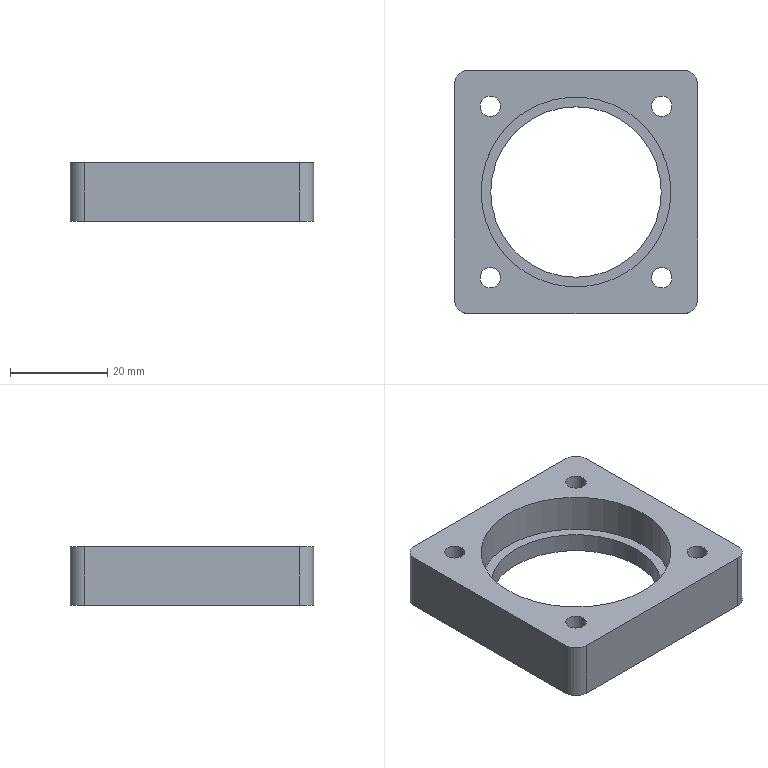Part | 1 solid | 23 faces | box 50 x 50 x 12 mm | volume 15837 mm3 | cylinder 16 | plane 7 | commonest cylinder face diameters 4.2 x8 6 x4 35 x2 39 x2
STEP:
#1=CARTESIAN_POINT('',(15.5,49.,-8.));
#2=VERTEX_POINT('',#1);
#3=CARTESIAN_POINT('',(54.5,49.,-8.));
#4=VERTEX_POINT('',#3);
#5=CARTESIAN_POINT('',(35.,49.,-8.));
#6=DIRECTION('',(0.,0.,1.));
#7=DIRECTION('',(1.,0.,0.));
#8=AXIS2_PLACEMENT_3D('',#5,#6,#7);
#9=CIRCLE('',#8,19.5);
#10=EDGE_CURVE('',#2,#4,#9,.T.);
#11=ORIENTED_EDGE('',*,*,#10,.F.);
#12=CARTESIAN_POINT('',(15.5,49.,0.));
#13=VERTEX_POINT('',#12);
#14=CARTESIAN_POINT('',(15.5,49.,-8.));
#15=DIRECTION('',(0.,0.,1.));
#16=VECTOR('',#15,1000.);
#17=LINE('',#14,#16);
#18=EDGE_CURVE('',#2,#13,#17,.T.);
#19=ORIENTED_EDGE('',*,*,#18,.T.);
#20=CARTESIAN_POINT('',(54.5,49.,0.));
#21=VERTEX_POINT('',#20);
#22=CARTESIAN_POINT('',(35.,49.,0.));
#23=DIRECTION('',(0.,0.,1.));
#24=DIRECTION('',(1.,0.,0.));
#25=AXIS2_PLACEMENT_3D('',#22,#23,#24);
#26=CIRCLE('',#25,19.5);
#27=EDGE_CURVE('',#13,#21,#26,.T.);
#28=ORIENTED_EDGE('',*,*,#27,.T.);
#29=CARTESIAN_POINT('',(54.5,49.,-8.));
#30=DIRECTION('',(0.,0.,1.));
#31=VECTOR('',#30,1000.);
#32=LINE('',#29,#31);
#33=EDGE_CURVE('',#4,#21,#32,.T.);
#34=ORIENTED_EDGE('',*,*,#33,.F.);
#35=EDGE_LOOP('',(#11,#19,#28,#34));
#36=FACE_OUTER_BOUND('',#35,.T.);
#37=CARTESIAN_POINT('',(35.,49.,-8.));
#38=DIRECTION('',(0.,0.,1.));
#39=DIRECTION('',(1.,0.,0.));
#40=AXIS2_PLACEMENT_3D('',#37,#38,#39);
#41=CYLINDRICAL_SURFACE('',#40,19.5);
#42=ADVANCED_FACE('',(#36),#41,.F.);
#43=CARTESIAN_POINT('',(19.497,66.604,-12.));
#44=VERTEX_POINT('',#43);
#45=CARTESIAN_POINT('',(15.297,66.604,-12.));
#46=VERTEX_POINT('',#45);
#47=CARTESIAN_POINT('',(17.397,66.604,-12.));
#48=DIRECTION('',(0.,0.,-1.));
#49=DIRECTION('',(1.,0.,0.));
#50=AXIS2_PLACEMENT_3D('',#47,#48,#49);
#51=CIRCLE('',#50,2.1);
#52=EDGE_CURVE('',#44,#46,#51,.T.);
#53=ORIENTED_EDGE('',*,*,#52,.T.);
#54=CARTESIAN_POINT('',(15.297,66.604,0.));
#55=VERTEX_POINT('',#54);
#56=CARTESIAN_POINT('',(15.297,66.604,0.));
#57=DIRECTION('',(0.,0.,1.));
#58=VECTOR('',#57,1000.);
#59=LINE('',#56,#58);
#60=EDGE_CURVE('',#46,#55,#59,.T.);
#61=ORIENTED_EDGE('',*,*,#60,.T.);
#62=CARTESIAN_POINT('',(19.497,66.604,0.));
#63=VERTEX_POINT('',#62);
#64=CARTESIAN_POINT('',(17.397,66.604,0.));
#65=DIRECTION('',(0.,0.,1.));
#66=DIRECTION('',(1.,0.,0.));
#67=AXIS2_PLACEMENT_3D('',#64,#65,#66);
#68=CIRCLE('',#67,2.1);
#69=EDGE_CURVE('',#55,#63,#68,.T.);
#70=ORIENTED_EDGE('',*,*,#69,.T.);
#71=CARTESIAN_POINT('',(19.497,66.604,0.));
#72=DIRECTION('',(0.,0.,1.));
#73=VECTOR('',#72,1000.);
#74=LINE('',#71,#73);
#75=EDGE_CURVE('',#44,#63,#74,.T.);
#76=ORIENTED_EDGE('',*,*,#75,.F.);
#77=EDGE_LOOP('',(#53,#61,#70,#76));
#78=FACE_OUTER_BOUND('',#77,.T.);
#79=CARTESIAN_POINT('',(17.397,66.604,0.));
#80=DIRECTION('',(0.,0.,1.));
#81=DIRECTION('',(1.,0.,0.));
#82=AXIS2_PLACEMENT_3D('',#79,#80,#81);
#83=CYLINDRICAL_SURFACE('',#82,2.1);
#84=ADVANCED_FACE('',(#78),#83,.F.);
#85=CARTESIAN_POINT('',(54.704,66.603,-12.));
#86=VERTEX_POINT('',#85);
#87=CARTESIAN_POINT('',(50.504,66.603,-12.));
#88=VERTEX_POINT('',#87);
#89=CARTESIAN_POINT('',(52.604,66.603,-12.));
#90=DIRECTION('',(0.,0.,-1.));
#91=DIRECTION('',(1.,0.,0.));
#92=AXIS2_PLACEMENT_3D('',#89,#90,#91);
#93=CIRCLE('',#92,2.1);
#94=EDGE_CURVE('',#86,#88,#93,.T.);
#95=ORIENTED_EDGE('',*,*,#94,.T.);
#96=CARTESIAN_POINT('',(50.504,66.603,0.));
#97=VERTEX_POINT('',#96);
#98=CARTESIAN_POINT('',(50.504,66.603,0.));
#99=DIRECTION('',(0.,0.,1.));
#100=VECTOR('',#99,1000.);
#101=LINE('',#98,#100);
#102=EDGE_CURVE('',#88,#97,#101,.T.);
#103=ORIENTED_EDGE('',*,*,#102,.T.);
#104=CARTESIAN_POINT('',(54.704,66.603,0.));
#105=VERTEX_POINT('',#104);
#106=CARTESIAN_POINT('',(52.604,66.603,0.));
#107=DIRECTION('',(0.,0.,1.));
#108=DIRECTION('',(1.,0.,0.));
#109=AXIS2_PLACEMENT_3D('',#106,#107,#108);
#110=CIRCLE('',#109,2.1);
#111=EDGE_CURVE('',#97,#105,#110,.T.);
#112=ORIENTED_EDGE('',*,*,#111,.T.);
#113=CARTESIAN_POINT('',(54.704,66.603,0.));
#114=DIRECTION('',(0.,0.,1.));
#115=VECTOR('',#114,1000.);
#116=LINE('',#113,#115);
#117=EDGE_CURVE('',#86,#105,#116,.T.);
#118=ORIENTED_EDGE('',*,*,#117,.F.);
#119=EDGE_LOOP('',(#95,#103,#112,#118));
#120=FACE_OUTER_BOUND('',#119,.T.);
#121=CARTESIAN_POINT('',(52.604,66.603,0.));
#122=DIRECTION('',(0.,0.,1.));
#123=DIRECTION('',(1.,0.,0.));
#124=AXIS2_PLACEMENT_3D('',#121,#122,#123);
#125=CYLINDRICAL_SURFACE('',#124,2.1);
#126=ADVANCED_FACE('',(#120),#125,.F.);
#127=CARTESIAN_POINT('',(54.703,31.396,-12.));
#128=VERTEX_POINT('',#127);
#129=CARTESIAN_POINT('',(50.503,31.396,-12.));
#130=VERTEX_POINT('',#129);
#131=CARTESIAN_POINT('',(52.603,31.396,-12.));
#132=DIRECTION('',(0.,0.,-1.));
#133=DIRECTION('',(1.,0.,0.));
#134=AXIS2_PLACEMENT_3D('',#131,#132,#133);
#135=CIRCLE('',#134,2.1);
#136=EDGE_CURVE('',#128,#130,#135,.T.);
#137=ORIENTED_EDGE('',*,*,#136,.T.);
#138=CARTESIAN_POINT('',(50.503,31.396,0.));
#139=VERTEX_POINT('',#138);
#140=CARTESIAN_POINT('',(50.503,31.396,0.));
#141=DIRECTION('',(0.,0.,1.));
#142=VECTOR('',#141,1000.);
#143=LINE('',#140,#142);
#144=EDGE_CURVE('',#130,#139,#143,.T.);
#145=ORIENTED_EDGE('',*,*,#144,.T.);
#146=CARTESIAN_POINT('',(54.703,31.396,0.));
#147=VERTEX_POINT('',#146);
#148=CARTESIAN_POINT('',(52.603,31.396,0.));
#149=DIRECTION('',(0.,0.,1.));
#150=DIRECTION('',(1.,0.,0.));
#151=AXIS2_PLACEMENT_3D('',#148,#149,#150);
#152=CIRCLE('',#151,2.1);
#153=EDGE_CURVE('',#139,#147,#152,.T.);
#154=ORIENTED_EDGE('',*,*,#153,.T.);
#155=CARTESIAN_POINT('',(54.703,31.396,0.));
#156=DIRECTION('',(0.,0.,1.));
#157=VECTOR('',#156,1000.);
#158=LINE('',#155,#157);
#159=EDGE_CURVE('',#128,#147,#158,.T.);
#160=ORIENTED_EDGE('',*,*,#159,.F.);
#161=EDGE_LOOP('',(#137,#145,#154,#160));
#162=FACE_OUTER_BOUND('',#161,.T.);
#163=CARTESIAN_POINT('',(52.603,31.396,0.));
#164=DIRECTION('',(0.,0.,1.));
#165=DIRECTION('',(1.,0.,0.));
#166=AXIS2_PLACEMENT_3D('',#163,#164,#165);
#167=CYLINDRICAL_SURFACE('',#166,2.1);
#168=ADVANCED_FACE('',(#162),#167,.F.);
#169=CARTESIAN_POINT('',(19.496,31.397,-12.));
#170=VERTEX_POINT('',#169);
#171=CARTESIAN_POINT('',(15.296,31.397,-12.));
#172=VERTEX_POINT('',#171);
#173=CARTESIAN_POINT('',(17.396,31.397,-12.));
#174=DIRECTION('',(0.,0.,-1.));
#175=DIRECTION('',(1.,0.,0.));
#176=AXIS2_PLACEMENT_3D('',#173,#174,#175);
#177=CIRCLE('',#176,2.1);
#178=EDGE_CURVE('',#170,#172,#177,.T.);
#179=ORIENTED_EDGE('',*,*,#178,.T.);
#180=CARTESIAN_POINT('',(15.296,31.397,0.));
#181=VERTEX_POINT('',#180);
#182=CARTESIAN_POINT('',(15.296,31.397,0.));
#183=DIRECTION('',(0.,0.,1.));
#184=VECTOR('',#183,1000.);
#185=LINE('',#182,#184);
#186=EDGE_CURVE('',#172,#181,#185,.T.);
#187=ORIENTED_EDGE('',*,*,#186,.T.);
#188=CARTESIAN_POINT('',(19.496,31.397,0.));
#189=VERTEX_POINT('',#188);
#190=CARTESIAN_POINT('',(17.396,31.397,0.));
#191=DIRECTION('',(0.,0.,1.));
#192=DIRECTION('',(1.,0.,0.));
#193=AXIS2_PLACEMENT_3D('',#190,#191,#192);
#194=CIRCLE('',#193,2.1);
#195=EDGE_CURVE('',#181,#189,#194,.T.);
#196=ORIENTED_EDGE('',*,*,#195,.T.);
#197=CARTESIAN_POINT('',(19.496,31.397,0.));
#198=DIRECTION('',(0.,0.,1.));
#199=VECTOR('',#198,1000.);
#200=LINE('',#197,#199);
#201=EDGE_CURVE('',#170,#189,#200,.T.);
#202=ORIENTED_EDGE('',*,*,#201,.F.);
#203=EDGE_LOOP('',(#179,#187,#196,#202));
#204=FACE_OUTER_BOUND('',#203,.T.);
#205=CARTESIAN_POINT('',(17.396,31.397,0.));
#206=DIRECTION('',(0.,0.,1.));
#207=DIRECTION('',(1.,0.,0.));
#208=AXIS2_PLACEMENT_3D('',#205,#206,#207);
#209=CYLINDRICAL_SURFACE('',#208,2.1);
#210=ADVANCED_FACE('',(#204),#209,.F.);
#211=CARTESIAN_POINT('',(52.5,49.,-12.));
#212=VERTEX_POINT('',#211);
#213=CARTESIAN_POINT('',(17.5,49.,-12.));
#214=VERTEX_POINT('',#213);
#215=CARTESIAN_POINT('',(35.,49.,-12.));
#216=DIRECTION('',(0.,0.,-1.));
#217=DIRECTION('',(1.,0.,0.));
#218=AXIS2_PLACEMENT_3D('',#215,#216,#217);
#219=CIRCLE('',#218,17.5);
#220=EDGE_CURVE('',#212,#214,#219,.T.);
#221=ORIENTED_EDGE('',*,*,#220,.T.);
#222=CARTESIAN_POINT('',(17.5,49.,-8.));
#223=VERTEX_POINT('',#222);
#224=CARTESIAN_POINT('',(17.5,49.,-20.));
#225=DIRECTION('',(0.,0.,1.));
#226=VECTOR('',#225,1000.);
#227=LINE('',#224,#226);
#228=EDGE_CURVE('',#214,#223,#227,.T.);
#229=ORIENTED_EDGE('',*,*,#228,.T.);
#230=CARTESIAN_POINT('',(52.5,49.,-8.));
#231=VERTEX_POINT('',#230);
#232=CARTESIAN_POINT('',(35.,49.,-8.));
#233=DIRECTION('',(0.,0.,-1.));
#234=DIRECTION('',(1.,0.,0.));
#235=AXIS2_PLACEMENT_3D('',#232,#233,#234);
#236=CIRCLE('',#235,17.5);
#237=EDGE_CURVE('',#231,#223,#236,.T.);
#238=ORIENTED_EDGE('',*,*,#237,.F.);
#239=CARTESIAN_POINT('',(52.5,49.,-20.));
#240=DIRECTION('',(0.,0.,1.));
#241=VECTOR('',#240,1000.);
#242=LINE('',#239,#241);
#243=EDGE_CURVE('',#212,#231,#242,.T.);
#244=ORIENTED_EDGE('',*,*,#243,.F.);
#245=EDGE_LOOP('',(#221,#229,#238,#244));
#246=FACE_OUTER_BOUND('',#245,.T.);
#247=CARTESIAN_POINT('',(35.,49.,-20.));
#248=DIRECTION('',(0.,0.,1.));
#249=DIRECTION('',(1.,0.,0.));
#250=AXIS2_PLACEMENT_3D('',#247,#248,#249);
#251=CYLINDRICAL_SURFACE('',#250,17.5);
#252=ADVANCED_FACE('',(#246),#251,.F.);
#253=ORIENTED_EDGE('',*,*,#228,.F.);
#254=CARTESIAN_POINT('',(35.,49.,-12.));
#255=DIRECTION('',(0.,0.,-1.));
#256=DIRECTION('',(1.,0.,0.));
#257=AXIS2_PLACEMENT_3D('',#254,#255,#256);
#258=CIRCLE('',#257,17.5);
#259=EDGE_CURVE('',#214,#212,#258,.T.);
#260=ORIENTED_EDGE('',*,*,#259,.T.);
#261=ORIENTED_EDGE('',*,*,#243,.T.);
#262=CARTESIAN_POINT('',(35.,49.,-8.));
#263=DIRECTION('',(0.,0.,-1.));
#264=DIRECTION('',(1.,0.,0.));
#265=AXIS2_PLACEMENT_3D('',#262,#263,#264);
#266=CIRCLE('',#265,17.5);
#267=EDGE_CURVE('',#223,#231,#266,.T.);
#268=ORIENTED_EDGE('',*,*,#267,.F.);
#269=EDGE_LOOP('',(#253,#260,#261,#268));
#270=FACE_OUTER_BOUND('',#269,.T.);
#271=CARTESIAN_POINT('',(35.,49.,-20.));
#272=DIRECTION('',(0.,0.,1.));
#273=DIRECTION('',(1.,0.,0.));
#274=AXIS2_PLACEMENT_3D('',#271,#272,#273);
#275=CYLINDRICAL_SURFACE('',#274,17.5);
#276=ADVANCED_FACE('',(#270),#275,.F.);
#277=CARTESIAN_POINT('',(35.,49.,0.));
#278=DIRECTION('',(0.,0.,1.));
#279=DIRECTION('',(1.,0.,0.));
#280=AXIS2_PLACEMENT_3D('',#277,#278,#279);
#281=CIRCLE('',#280,19.5);
#282=EDGE_CURVE('',#21,#13,#281,.T.);
#283=ORIENTED_EDGE('',*,*,#282,.F.);
#284=ORIENTED_EDGE('',*,*,#27,.F.);
#285=EDGE_LOOP('',(#283,#284));
#286=FACE_BOUND('',#285,.T.);
#287=CARTESIAN_POINT('',(17.396,31.397,0.));
#288=DIRECTION('',(0.,0.,1.));
#289=DIRECTION('',(1.,0.,0.));
#290=AXIS2_PLACEMENT_3D('',#287,#288,#289);
#291=CIRCLE('',#290,2.1);
#292=EDGE_CURVE('',#189,#181,#291,.T.);
#293=ORIENTED_EDGE('',*,*,#292,.F.);
#294=ORIENTED_EDGE('',*,*,#195,.F.);
#295=EDGE_LOOP('',(#293,#294));
#296=FACE_BOUND('',#295,.T.);
#297=CARTESIAN_POINT('',(52.603,31.396,0.));
#298=DIRECTION('',(0.,0.,1.));
#299=DIRECTION('',(1.,0.,0.));
#300=AXIS2_PLACEMENT_3D('',#297,#298,#299);
#301=CIRCLE('',#300,2.1);
#302=EDGE_CURVE('',#147,#139,#301,.T.);
#303=ORIENTED_EDGE('',*,*,#302,.F.);
#304=ORIENTED_EDGE('',*,*,#153,.F.);
#305=EDGE_LOOP('',(#303,#304));
#306=FACE_BOUND('',#305,.T.);
#307=CARTESIAN_POINT('',(52.604,66.603,0.));
#308=DIRECTION('',(0.,0.,1.));
#309=DIRECTION('',(1.,0.,0.));
#310=AXIS2_PLACEMENT_3D('',#307,#308,#309);
#311=CIRCLE('',#310,2.1);
#312=EDGE_CURVE('',#105,#97,#311,.T.);
#313=ORIENTED_EDGE('',*,*,#312,.F.);
#314=ORIENTED_EDGE('',*,*,#111,.F.);
#315=EDGE_LOOP('',(#313,#314));
#316=FACE_BOUND('',#315,.T.);
#317=CARTESIAN_POINT('',(17.397,66.604,0.));
#318=DIRECTION('',(0.,0.,1.));
#319=DIRECTION('',(1.,0.,0.));
#320=AXIS2_PLACEMENT_3D('',#317,#318,#319);
#321=CIRCLE('',#320,2.1);
#322=EDGE_CURVE('',#63,#55,#321,.T.);
#323=ORIENTED_EDGE('',*,*,#322,.F.);
#324=ORIENTED_EDGE('',*,*,#69,.F.);
#325=EDGE_LOOP('',(#323,#324));
#326=FACE_BOUND('',#325,.T.);
#327=CARTESIAN_POINT('',(10.,71.,0.));
#328=VERTEX_POINT('',#327);
#329=CARTESIAN_POINT('',(10.,27.,0.));
#330=VERTEX_POINT('',#329);
#331=CARTESIAN_POINT('',(10.,71.,0.));
#332=DIRECTION('',(0.,-1.,0.));
#333=VECTOR('',#332,1000.);
#334=LINE('',#331,#333);
#335=EDGE_CURVE('',#328,#330,#334,.T.);
#336=ORIENTED_EDGE('',*,*,#335,.T.);
#337=CARTESIAN_POINT('',(13.,24.,0.));
#338=VERTEX_POINT('',#337);
#339=CARTESIAN_POINT('',(13.,27.,0.));
#340=DIRECTION('',(0.,0.,1.));
#341=DIRECTION('',(1.,0.,0.));
#342=AXIS2_PLACEMENT_3D('',#339,#340,#341);
#343=CIRCLE('',#342,3.);
#344=EDGE_CURVE('',#330,#338,#343,.T.);
#345=ORIENTED_EDGE('',*,*,#344,.T.);
#346=CARTESIAN_POINT('',(57.,24.,0.));
#347=VERTEX_POINT('',#346);
#348=CARTESIAN_POINT('',(13.,24.,0.));
#349=DIRECTION('',(1.,0.,0.));
#350=VECTOR('',#349,1000.);
#351=LINE('',#348,#350);
#352=EDGE_CURVE('',#338,#347,#351,.T.);
#353=ORIENTED_EDGE('',*,*,#352,.T.);
#354=CARTESIAN_POINT('',(60.,27.,0.));
#355=VERTEX_POINT('',#354);
#356=CARTESIAN_POINT('',(57.,27.,0.));
#357=DIRECTION('',(0.,0.,1.));
#358=DIRECTION('',(1.,0.,0.));
#359=AXIS2_PLACEMENT_3D('',#356,#357,#358);
#360=CIRCLE('',#359,3.);
#361=EDGE_CURVE('',#347,#355,#360,.T.);
#362=ORIENTED_EDGE('',*,*,#361,.T.);
#363=CARTESIAN_POINT('',(60.,71.,0.));
#364=VERTEX_POINT('',#363);
#365=CARTESIAN_POINT('',(60.,71.,0.));
#366=DIRECTION('',(0.,1.,0.));
#367=VECTOR('',#366,1000.);
#368=LINE('',#365,#367);
#369=EDGE_CURVE('',#355,#364,#368,.T.);
#370=ORIENTED_EDGE('',*,*,#369,.T.);
#371=CARTESIAN_POINT('',(57.,74.,0.));
#372=VERTEX_POINT('',#371);
#373=CARTESIAN_POINT('',(57.,71.,0.));
#374=DIRECTION('',(0.,0.,1.));
#375=DIRECTION('',(-1.,0.,0.));
#376=AXIS2_PLACEMENT_3D('',#373,#374,#375);
#377=CIRCLE('',#376,3.);
#378=EDGE_CURVE('',#364,#372,#377,.T.);
#379=ORIENTED_EDGE('',*,*,#378,.T.);
#380=CARTESIAN_POINT('',(13.,74.,0.));
#381=VERTEX_POINT('',#380);
#382=CARTESIAN_POINT('',(13.,74.,0.));
#383=DIRECTION('',(-1.,0.,0.));
#384=VECTOR('',#383,1000.);
#385=LINE('',#382,#384);
#386=EDGE_CURVE('',#372,#381,#385,.T.);
#387=ORIENTED_EDGE('',*,*,#386,.T.);
#388=CARTESIAN_POINT('',(13.,71.,0.));
#389=DIRECTION('',(0.,0.,1.));
#390=DIRECTION('',(1.,0.,0.));
#391=AXIS2_PLACEMENT_3D('',#388,#389,#390);
#392=CIRCLE('',#391,3.);
#393=EDGE_CURVE('',#381,#328,#392,.T.);
#394=ORIENTED_EDGE('',*,*,#393,.T.);
#395=EDGE_LOOP('',(#336,#345,#353,#362,#370,#379,#387,#394));
#396=FACE_OUTER_BOUND('',#395,.T.);
#397=CARTESIAN_POINT('',(0.,0.,0.));
#398=DIRECTION('',(0.,0.,1.));
#399=DIRECTION('',(1.,0.,0.));
#400=AXIS2_PLACEMENT_3D('',#397,#398,#399);
#401=PLANE('',#400);
#402=ADVANCED_FACE('',(#286,#296,#306,#316,#326,#396),#401,.T.);
#403=ORIENTED_EDGE('',*,*,#186,.F.);
#404=CARTESIAN_POINT('',(17.396,31.397,-12.));
#405=DIRECTION('',(0.,0.,-1.));
#406=DIRECTION('',(1.,0.,0.));
#407=AXIS2_PLACEMENT_3D('',#404,#405,#406);
#408=CIRCLE('',#407,2.1);
#409=EDGE_CURVE('',#172,#170,#408,.T.);
#410=ORIENTED_EDGE('',*,*,#409,.T.);
#411=ORIENTED_EDGE('',*,*,#201,.T.);
#412=ORIENTED_EDGE('',*,*,#292,.T.);
#413=EDGE_LOOP('',(#403,#410,#411,#412));
#414=FACE_OUTER_BOUND('',#413,.T.);
#415=CARTESIAN_POINT('',(17.396,31.397,0.));
#416=DIRECTION('',(0.,0.,1.));
#417=DIRECTION('',(1.,0.,0.));
#418=AXIS2_PLACEMENT_3D('',#415,#416,#417);
#419=CYLINDRICAL_SURFACE('',#418,2.1);
#420=ADVANCED_FACE('',(#414),#419,.F.);
#421=ORIENTED_EDGE('',*,*,#144,.F.);
#422=CARTESIAN_POINT('',(52.603,31.396,-12.));
#423=DIRECTION('',(0.,0.,-1.));
#424=DIRECTION('',(1.,0.,0.));
#425=AXIS2_PLACEMENT_3D('',#422,#423,#424);
#426=CIRCLE('',#425,2.1);
#427=EDGE_CURVE('',#130,#128,#426,.T.);
#428=ORIENTED_EDGE('',*,*,#427,.T.);
#429=ORIENTED_EDGE('',*,*,#159,.T.);
#430=ORIENTED_EDGE('',*,*,#302,.T.);
#431=EDGE_LOOP('',(#421,#428,#429,#430));
#432=FACE_OUTER_BOUND('',#431,.T.);
#433=CARTESIAN_POINT('',(52.603,31.396,0.));
#434=DIRECTION('',(0.,0.,1.));
#435=DIRECTION('',(1.,0.,0.));
#436=AXIS2_PLACEMENT_3D('',#433,#434,#435);
#437=CYLINDRICAL_SURFACE('',#436,2.1);
#438=ADVANCED_FACE('',(#432),#437,.F.);
#439=ORIENTED_EDGE('',*,*,#102,.F.);
#440=CARTESIAN_POINT('',(52.604,66.603,-12.));
#441=DIRECTION('',(0.,0.,-1.));
#442=DIRECTION('',(1.,0.,0.));
#443=AXIS2_PLACEMENT_3D('',#440,#441,#442);
#444=CIRCLE('',#443,2.1);
#445=EDGE_CURVE('',#88,#86,#444,.T.);
#446=ORIENTED_EDGE('',*,*,#445,.T.);
#447=ORIENTED_EDGE('',*,*,#117,.T.);
#448=ORIENTED_EDGE('',*,*,#312,.T.);
#449=EDGE_LOOP('',(#439,#446,#447,#448));
#450=FACE_OUTER_BOUND('',#449,.T.);
#451=CARTESIAN_POINT('',(52.604,66.603,0.));
#452=DIRECTION('',(0.,0.,1.));
#453=DIRECTION('',(1.,0.,0.));
#454=AXIS2_PLACEMENT_3D('',#451,#452,#453);
#455=CYLINDRICAL_SURFACE('',#454,2.1);
#456=ADVANCED_FACE('',(#450),#455,.F.);
#457=ORIENTED_EDGE('',*,*,#60,.F.);
#458=CARTESIAN_POINT('',(17.397,66.604,-12.));
#459=DIRECTION('',(0.,0.,-1.));
#460=DIRECTION('',(1.,0.,0.));
#461=AXIS2_PLACEMENT_3D('',#458,#459,#460);
#462=CIRCLE('',#461,2.1);
#463=EDGE_CURVE('',#46,#44,#462,.T.);
#464=ORIENTED_EDGE('',*,*,#463,.T.);
#465=ORIENTED_EDGE('',*,*,#75,.T.);
#466=ORIENTED_EDGE('',*,*,#322,.T.);
#467=EDGE_LOOP('',(#457,#464,#465,#466));
#468=FACE_OUTER_BOUND('',#467,.T.);
#469=CARTESIAN_POINT('',(17.397,66.604,0.));
#470=DIRECTION('',(0.,0.,1.));
#471=DIRECTION('',(1.,0.,0.));
#472=AXIS2_PLACEMENT_3D('',#469,#470,#471);
#473=CYLINDRICAL_SURFACE('',#472,2.1);
#474=ADVANCED_FACE('',(#468),#473,.F.);
#475=CARTESIAN_POINT('',(13.,24.,-12.));
#476=VERTEX_POINT('',#475);
#477=CARTESIAN_POINT('',(10.,27.,-12.));
#478=VERTEX_POINT('',#477);
#479=CARTESIAN_POINT('',(13.,27.,-12.));
#480=DIRECTION('',(0.,0.,-1.));
#481=DIRECTION('',(1.,0.,0.));
#482=AXIS2_PLACEMENT_3D('',#479,#480,#481);
#483=CIRCLE('',#482,3.);
#484=EDGE_CURVE('',#476,#478,#483,.T.);
#485=ORIENTED_EDGE('',*,*,#484,.F.);
#486=CARTESIAN_POINT('',(13.,24.,-20.));
#487=DIRECTION('',(0.,0.,1.));
#488=VECTOR('',#487,1000.);
#489=LINE('',#486,#488);
#490=EDGE_CURVE('',#476,#338,#489,.T.);
#491=ORIENTED_EDGE('',*,*,#490,.T.);
#492=ORIENTED_EDGE('',*,*,#344,.F.);
#493=CARTESIAN_POINT('',(10.,27.,-20.));
#494=DIRECTION('',(0.,0.,1.));
#495=VECTOR('',#494,1000.);
#496=LINE('',#493,#495);
#497=EDGE_CURVE('',#478,#330,#496,.T.);
#498=ORIENTED_EDGE('',*,*,#497,.F.);
#499=EDGE_LOOP('',(#485,#491,#492,#498));
#500=FACE_OUTER_BOUND('',#499,.T.);
#501=CARTESIAN_POINT('',(13.,27.,-20.));
#502=DIRECTION('',(0.,0.,1.));
#503=DIRECTION('',(1.,0.,0.));
#504=AXIS2_PLACEMENT_3D('',#501,#502,#503);
#505=CYLINDRICAL_SURFACE('',#504,3.);
#506=ADVANCED_FACE('',(#500),#505,.T.);
#507=CARTESIAN_POINT('',(10.,71.,-12.));
#508=VERTEX_POINT('',#507);
#509=CARTESIAN_POINT('',(10.,24.,-12.));
#510=DIRECTION('',(0.,1.,0.));
#511=VECTOR('',#510,1000.);
#512=LINE('',#509,#511);
#513=EDGE_CURVE('',#478,#508,#512,.T.);
#514=ORIENTED_EDGE('',*,*,#513,.F.);
#515=ORIENTED_EDGE('',*,*,#497,.T.);
#516=ORIENTED_EDGE('',*,*,#335,.F.);
#517=CARTESIAN_POINT('',(10.,71.,-20.));
#518=DIRECTION('',(0.,0.,1.));
#519=VECTOR('',#518,1000.);
#520=LINE('',#517,#519);
#521=EDGE_CURVE('',#508,#328,#520,.T.);
#522=ORIENTED_EDGE('',*,*,#521,.F.);
#523=EDGE_LOOP('',(#514,#515,#516,#522));
#524=FACE_OUTER_BOUND('',#523,.T.);
#525=CARTESIAN_POINT('',(10.,71.,-20.));
#526=DIRECTION('',(-1.,0.,0.));
#527=DIRECTION('',(0.,-1.,0.));
#528=AXIS2_PLACEMENT_3D('',#525,#526,#527);
#529=PLANE('',#528);
#530=ADVANCED_FACE('',(#524),#529,.T.);
#531=CARTESIAN_POINT('',(13.,74.,-12.));
#532=VERTEX_POINT('',#531);
#533=CARTESIAN_POINT('',(13.,71.,-12.));
#534=DIRECTION('',(0.,0.,-1.));
#535=DIRECTION('',(1.,0.,0.));
#536=AXIS2_PLACEMENT_3D('',#533,#534,#535);
#537=CIRCLE('',#536,3.);
#538=EDGE_CURVE('',#508,#532,#537,.T.);
#539=ORIENTED_EDGE('',*,*,#538,.F.);
#540=ORIENTED_EDGE('',*,*,#521,.T.);
#541=ORIENTED_EDGE('',*,*,#393,.F.);
#542=CARTESIAN_POINT('',(13.,74.,-20.));
#543=DIRECTION('',(0.,0.,1.));
#544=VECTOR('',#543,1000.);
#545=LINE('',#542,#544);
#546=EDGE_CURVE('',#532,#381,#545,.T.);
#547=ORIENTED_EDGE('',*,*,#546,.F.);
#548=EDGE_LOOP('',(#539,#540,#541,#547));
#549=FACE_OUTER_BOUND('',#548,.T.);
#550=CARTESIAN_POINT('',(13.,71.,-20.));
#551=DIRECTION('',(0.,0.,1.));
#552=DIRECTION('',(1.,0.,0.));
#553=AXIS2_PLACEMENT_3D('',#550,#551,#552);
#554=CYLINDRICAL_SURFACE('',#553,3.);
#555=ADVANCED_FACE('',(#549),#554,.T.);
#556=CARTESIAN_POINT('',(57.,74.,-12.));
#557=VERTEX_POINT('',#556);
#558=CARTESIAN_POINT('',(10.,74.,-12.));
#559=DIRECTION('',(1.,0.,0.));
#560=VECTOR('',#559,1000.);
#561=LINE('',#558,#560);
#562=EDGE_CURVE('',#532,#557,#561,.T.);
#563=ORIENTED_EDGE('',*,*,#562,.F.);
#564=ORIENTED_EDGE('',*,*,#546,.T.);
#565=ORIENTED_EDGE('',*,*,#386,.F.);
#566=CARTESIAN_POINT('',(57.,74.,-20.));
#567=DIRECTION('',(0.,0.,1.));
#568=VECTOR('',#567,1000.);
#569=LINE('',#566,#568);
#570=EDGE_CURVE('',#557,#372,#569,.T.);
#571=ORIENTED_EDGE('',*,*,#570,.F.);
#572=EDGE_LOOP('',(#563,#564,#565,#571));
#573=FACE_OUTER_BOUND('',#572,.T.);
#574=CARTESIAN_POINT('',(13.,74.,-20.));
#575=DIRECTION('',(0.,1.,0.));
#576=DIRECTION('',(0.,0.,1.));
#577=AXIS2_PLACEMENT_3D('',#574,#575,#576);
#578=PLANE('',#577);
#579=ADVANCED_FACE('',(#573),#578,.T.);
#580=CARTESIAN_POINT('',(60.,71.,-12.));
#581=VERTEX_POINT('',#580);
#582=CARTESIAN_POINT('',(57.,71.,-12.));
#583=DIRECTION('',(0.,0.,-1.));
#584=DIRECTION('',(1.,0.,0.));
#585=AXIS2_PLACEMENT_3D('',#582,#583,#584);
#586=CIRCLE('',#585,3.);
#587=EDGE_CURVE('',#557,#581,#586,.T.);
#588=ORIENTED_EDGE('',*,*,#587,.F.);
#589=ORIENTED_EDGE('',*,*,#570,.T.);
#590=ORIENTED_EDGE('',*,*,#378,.F.);
#591=CARTESIAN_POINT('',(60.,71.,-20.));
#592=DIRECTION('',(0.,0.,1.));
#593=VECTOR('',#592,1000.);
#594=LINE('',#591,#593);
#595=EDGE_CURVE('',#581,#364,#594,.T.);
#596=ORIENTED_EDGE('',*,*,#595,.F.);
#597=EDGE_LOOP('',(#588,#589,#590,#596));
#598=FACE_OUTER_BOUND('',#597,.T.);
#599=CARTESIAN_POINT('',(57.,71.,-20.));
#600=DIRECTION('',(0.,0.,1.));
#601=DIRECTION('',(1.,0.,0.));
#602=AXIS2_PLACEMENT_3D('',#599,#600,#601);
#603=CYLINDRICAL_SURFACE('',#602,3.);
#604=ADVANCED_FACE('',(#598),#603,.T.);
#605=CARTESIAN_POINT('',(60.,27.,-12.));
#606=VERTEX_POINT('',#605);
#607=CARTESIAN_POINT('',(60.,24.,-12.));
#608=DIRECTION('',(0.,1.,0.));
#609=VECTOR('',#608,1000.);
#610=LINE('',#607,#609);
#611=EDGE_CURVE('',#606,#581,#610,.T.);
#612=ORIENTED_EDGE('',*,*,#611,.T.);
#613=ORIENTED_EDGE('',*,*,#595,.T.);
#614=ORIENTED_EDGE('',*,*,#369,.F.);
#615=CARTESIAN_POINT('',(60.,27.,-20.));
#616=DIRECTION('',(0.,0.,1.));
#617=VECTOR('',#616,1000.);
#618=LINE('',#615,#617);
#619=EDGE_CURVE('',#606,#355,#618,.T.);
#620=ORIENTED_EDGE('',*,*,#619,.F.);
#621=EDGE_LOOP('',(#612,#613,#614,#620));
#622=FACE_OUTER_BOUND('',#621,.T.);
#623=CARTESIAN_POINT('',(60.,71.,-20.));
#624=DIRECTION('',(1.,0.,0.));
#625=DIRECTION('',(0.,1.,0.));
#626=AXIS2_PLACEMENT_3D('',#623,#624,#625);
#627=PLANE('',#626);
#628=ADVANCED_FACE('',(#622),#627,.T.);
#629=CARTESIAN_POINT('',(57.,24.,-12.));
#630=VERTEX_POINT('',#629);
#631=CARTESIAN_POINT('',(57.,27.,-12.));
#632=DIRECTION('',(0.,0.,-1.));
#633=DIRECTION('',(1.,0.,0.));
#634=AXIS2_PLACEMENT_3D('',#631,#632,#633);
#635=CIRCLE('',#634,3.);
#636=EDGE_CURVE('',#606,#630,#635,.T.);
#637=ORIENTED_EDGE('',*,*,#636,.F.);
#638=ORIENTED_EDGE('',*,*,#619,.T.);
#639=ORIENTED_EDGE('',*,*,#361,.F.);
#640=CARTESIAN_POINT('',(57.,24.,-20.));
#641=DIRECTION('',(0.,0.,1.));
#642=VECTOR('',#641,1000.);
#643=LINE('',#640,#642);
#644=EDGE_CURVE('',#630,#347,#643,.T.);
#645=ORIENTED_EDGE('',*,*,#644,.F.);
#646=EDGE_LOOP('',(#637,#638,#639,#645));
#647=FACE_OUTER_BOUND('',#646,.T.);
#648=CARTESIAN_POINT('',(57.,27.,-20.));
#649=DIRECTION('',(0.,0.,1.));
#650=DIRECTION('',(1.,0.,0.));
#651=AXIS2_PLACEMENT_3D('',#648,#649,#650);
#652=CYLINDRICAL_SURFACE('',#651,3.);
#653=ADVANCED_FACE('',(#647),#652,.T.);
#654=CARTESIAN_POINT('',(13.,24.,-12.));
#655=DIRECTION('',(-1.,0.,0.));
#656=VECTOR('',#655,1000.);
#657=LINE('',#654,#656);
#658=EDGE_CURVE('',#630,#476,#657,.T.);
#659=ORIENTED_EDGE('',*,*,#658,.F.);
#660=ORIENTED_EDGE('',*,*,#644,.T.);
#661=ORIENTED_EDGE('',*,*,#352,.F.);
#662=ORIENTED_EDGE('',*,*,#490,.F.);
#663=EDGE_LOOP('',(#659,#660,#661,#662));
#664=FACE_OUTER_BOUND('',#663,.T.);
#665=CARTESIAN_POINT('',(13.,24.,-20.));
#666=DIRECTION('',(0.,-1.,0.));
#667=DIRECTION('',(0.,0.,-1.));
#668=AXIS2_PLACEMENT_3D('',#665,#666,#667);
#669=PLANE('',#668);
#670=ADVANCED_FACE('',(#664),#669,.T.);
#671=ORIENTED_EDGE('',*,*,#178,.F.);
#672=ORIENTED_EDGE('',*,*,#409,.F.);
#673=EDGE_LOOP('',(#671,#672));
#674=FACE_BOUND('',#673,.T.);
#675=ORIENTED_EDGE('',*,*,#94,.F.);
#676=ORIENTED_EDGE('',*,*,#445,.F.);
#677=EDGE_LOOP('',(#675,#676));
#678=FACE_BOUND('',#677,.T.);
#679=ORIENTED_EDGE('',*,*,#484,.T.);
#680=ORIENTED_EDGE('',*,*,#513,.T.);
#681=ORIENTED_EDGE('',*,*,#538,.T.);
#682=ORIENTED_EDGE('',*,*,#562,.T.);
#683=ORIENTED_EDGE('',*,*,#587,.T.);
#684=ORIENTED_EDGE('',*,*,#611,.F.);
#685=ORIENTED_EDGE('',*,*,#636,.T.);
#686=ORIENTED_EDGE('',*,*,#658,.T.);
#687=EDGE_LOOP('',(#679,#680,#681,#682,#683,#684,#685,#686));
#688=FACE_OUTER_BOUND('',#687,.T.);
#689=ORIENTED_EDGE('',*,*,#52,.F.);
#690=ORIENTED_EDGE('',*,*,#463,.F.);
#691=EDGE_LOOP('',(#689,#690));
#692=FACE_BOUND('',#691,.T.);
#693=ORIENTED_EDGE('',*,*,#136,.F.);
#694=ORIENTED_EDGE('',*,*,#427,.F.);
#695=EDGE_LOOP('',(#693,#694));
#696=FACE_BOUND('',#695,.T.);
#697=ORIENTED_EDGE('',*,*,#220,.F.);
#698=ORIENTED_EDGE('',*,*,#259,.F.);
#699=EDGE_LOOP('',(#697,#698));
#700=FACE_BOUND('',#699,.T.);
#701=CARTESIAN_POINT('',(10.,24.,-12.));
#702=DIRECTION('',(0.,0.,1.));
#703=DIRECTION('',(1.,0.,0.));
#704=AXIS2_PLACEMENT_3D('',#701,#702,#703);
#705=PLANE('',#704);
#706=ADVANCED_FACE('',(#674,#678,#688,#692,#696,#700),#705,.F.);
#707=CARTESIAN_POINT('',(35.,49.,-8.));
#708=DIRECTION('',(0.,0.,1.));
#709=DIRECTION('',(1.,0.,0.));
#710=AXIS2_PLACEMENT_3D('',#707,#708,#709);
#711=CIRCLE('',#710,19.5);
#712=EDGE_CURVE('',#4,#2,#711,.T.);
#713=ORIENTED_EDGE('',*,*,#712,.T.);
#714=ORIENTED_EDGE('',*,*,#10,.T.);
#715=EDGE_LOOP('',(#713,#714));
#716=FACE_OUTER_BOUND('',#715,.T.);
#717=ORIENTED_EDGE('',*,*,#237,.T.);
#718=ORIENTED_EDGE('',*,*,#267,.T.);
#719=EDGE_LOOP('',(#717,#718));
#720=FACE_BOUND('',#719,.T.);
#721=CARTESIAN_POINT('',(35.,49.,-8.));
#722=DIRECTION('',(0.,0.,1.));
#723=DIRECTION('',(1.,0.,0.));
#724=AXIS2_PLACEMENT_3D('',#721,#722,#723);
#725=PLANE('',#724);
#726=ADVANCED_FACE('',(#716,#720),#725,.T.);
#727=ORIENTED_EDGE('',*,*,#18,.F.);
#728=ORIENTED_EDGE('',*,*,#712,.F.);
#729=ORIENTED_EDGE('',*,*,#33,.T.);
#730=ORIENTED_EDGE('',*,*,#282,.T.);
#731=EDGE_LOOP('',(#727,#728,#729,#730));
#732=FACE_OUTER_BOUND('',#731,.T.);
#733=CARTESIAN_POINT('',(35.,49.,-8.));
#734=DIRECTION('',(0.,0.,1.));
#735=DIRECTION('',(1.,0.,0.));
#736=AXIS2_PLACEMENT_3D('',#733,#734,#735);
#737=CYLINDRICAL_SURFACE('',#736,19.5);
#738=ADVANCED_FACE('',(#732),#737,.F.);
#739=CLOSED_SHELL('',(#42,#84,#126,#168,#210,#252,#276,#402,#420,#438,#456,#474,#506,#530,#555,#579,#604,#628,#653,#670,#706,#726,#738));
#740=MANIFOLD_SOLID_BREP('',#739);
#741=CARTESIAN_POINT('',(0.,0.,0.));
#742=DIRECTION('',(0.,0.,1.));
#743=DIRECTION('',(1.,0.,0.));
#744=AXIS2_PLACEMENT_3D('',#741,#742,#743);
#745=(LENGTH_UNIT()NAMED_UNIT(*)SI_UNIT(.MILLI.,.METRE.));
#746=UNCERTAINTY_MEASURE_WITH_UNIT(LENGTH_MEASURE(0.00001),#745,'','');
#747=(NAMED_UNIT(*)PLANE_ANGLE_UNIT()SI_UNIT($,.RADIAN.));
#748=(NAMED_UNIT(*)SI_UNIT($,.STERADIAN.)SOLID_ANGLE_UNIT());
#749=(GEOMETRIC_REPRESENTATION_CONTEXT(3)GLOBAL_UNCERTAINTY_ASSIGNED_CONTEXT((#746))GLOBAL_UNIT_ASSIGNED_CONTEXT((#745,#747,#748))REPRESENTATION_CONTEXT('',''));
#750=ADVANCED_BREP_SHAPE_REPRESENTATION('',(#740,#744),#749);